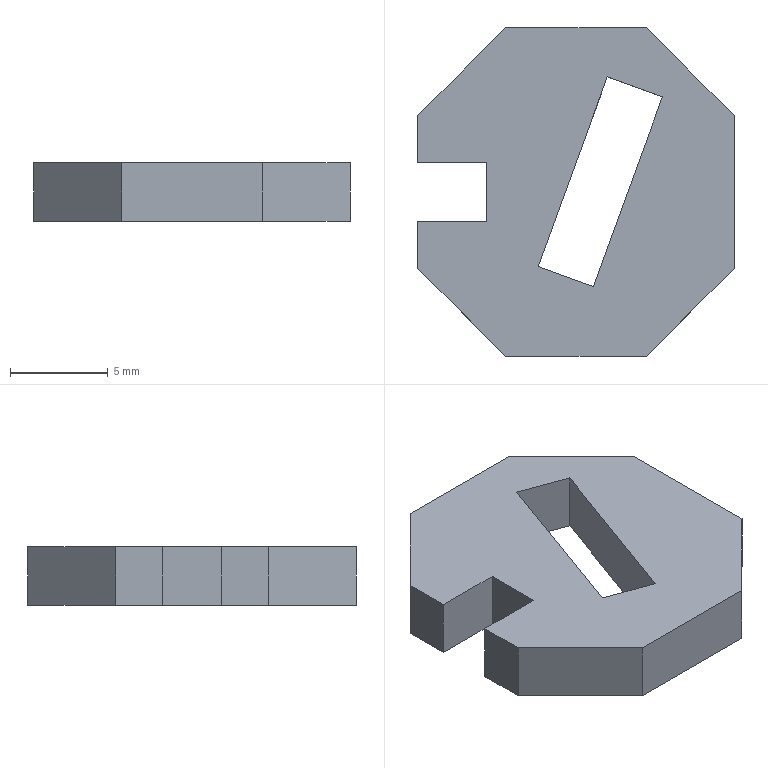Part | SolidWorks | features BaseBody 1 | 1 solid | 18 faces | box 16.185 x 16.813 x 3 mm | volume 570.375 mm3 | plane 18
STEP:
#1=CARTESIAN_POINT('',(11.966,25.62,-1.5));
#2=VERTEX_POINT('',#1);
#3=CARTESIAN_POINT('',(14.785,24.594,-1.5));
#4=VERTEX_POINT('',#3);
#5=CARTESIAN_POINT('',(14.785,24.594,-1.5));
#6=DIRECTION('',(0.9396,-0.3421,0.));
#7=VECTOR('',#6,1000.);
#8=LINE('',#5,#7);
#9=EDGE_CURVE('',#2,#4,#8,.T.);
#10=ORIENTED_EDGE('',*,*,#9,.F.);
#11=CARTESIAN_POINT('',(11.966,25.62,1.5));
#12=VERTEX_POINT('',#11);
#13=CARTESIAN_POINT('',(11.966,25.62,1.5));
#14=DIRECTION('',(0.,0.,-1.));
#15=VECTOR('',#14,1000.);
#16=LINE('',#13,#15);
#17=EDGE_CURVE('',#12,#2,#16,.T.);
#18=ORIENTED_EDGE('',*,*,#17,.F.);
#19=CARTESIAN_POINT('',(14.785,24.594,1.5));
#20=VERTEX_POINT('',#19);
#21=CARTESIAN_POINT('',(14.785,24.594,1.5));
#22=DIRECTION('',(0.9396,-0.3421,0.));
#23=VECTOR('',#22,1000.);
#24=LINE('',#21,#23);
#25=EDGE_CURVE('',#12,#20,#24,.T.);
#26=ORIENTED_EDGE('',*,*,#25,.T.);
#27=CARTESIAN_POINT('',(14.785,24.594,1.5));
#28=DIRECTION('',(0.,0.,-1.));
#29=VECTOR('',#28,1000.);
#30=LINE('',#27,#29);
#31=EDGE_CURVE('',#20,#4,#30,.T.);
#32=ORIENTED_EDGE('',*,*,#31,.T.);
#33=EDGE_LOOP('',(#10,#18,#26,#32));
#34=FACE_OUTER_BOUND('',#33,.T.);
#35=CARTESIAN_POINT('',(14.785,24.594,1.5));
#36=DIRECTION('',(0.3421,0.9396,0.));
#37=DIRECTION('',(0.,0.,-1.));
#38=AXIS2_PLACEMENT_3D('',#35,#36,#37);
#39=PLANE('',#38);
#40=ADVANCED_FACE('',(#34),#39,.T.);
#41=CARTESIAN_POINT('',(15.5,35.326,-1.5));
#42=VERTEX_POINT('',#41);
#43=CARTESIAN_POINT('',(11.966,25.62,-1.5));
#44=DIRECTION('',(-0.3421,-0.9396,0.));
#45=VECTOR('',#44,1000.);
#46=LINE('',#43,#45);
#47=EDGE_CURVE('',#42,#2,#46,.T.);
#48=ORIENTED_EDGE('',*,*,#47,.F.);
#49=CARTESIAN_POINT('',(15.5,35.326,1.5));
#50=VERTEX_POINT('',#49);
#51=CARTESIAN_POINT('',(15.5,35.326,1.5));
#52=DIRECTION('',(0.,0.,-1.));
#53=VECTOR('',#52,1000.);
#54=LINE('',#51,#53);
#55=EDGE_CURVE('',#50,#42,#54,.T.);
#56=ORIENTED_EDGE('',*,*,#55,.F.);
#57=CARTESIAN_POINT('',(11.966,25.62,1.5));
#58=DIRECTION('',(-0.3421,-0.9396,0.));
#59=VECTOR('',#58,1000.);
#60=LINE('',#57,#59);
#61=EDGE_CURVE('',#50,#12,#60,.T.);
#62=ORIENTED_EDGE('',*,*,#61,.T.);
#63=ORIENTED_EDGE('',*,*,#17,.T.);
#64=EDGE_LOOP('',(#48,#56,#62,#63));
#65=FACE_OUTER_BOUND('',#64,.T.);
#66=CARTESIAN_POINT('',(11.966,25.62,1.5));
#67=DIRECTION('',(0.9396,-0.3421,0.));
#68=DIRECTION('',(0.,0.,-1.));
#69=AXIS2_PLACEMENT_3D('',#66,#67,#68);
#70=PLANE('',#69);
#71=ADVANCED_FACE('',(#65),#70,.T.);
#72=CARTESIAN_POINT('',(18.319,34.3,-1.5));
#73=VERTEX_POINT('',#72);
#74=CARTESIAN_POINT('',(15.5,35.326,-1.5));
#75=DIRECTION('',(-0.9396,0.3421,0.));
#76=VECTOR('',#75,1000.);
#77=LINE('',#74,#76);
#78=EDGE_CURVE('',#73,#42,#77,.T.);
#79=ORIENTED_EDGE('',*,*,#78,.F.);
#80=CARTESIAN_POINT('',(18.319,34.3,1.5));
#81=VERTEX_POINT('',#80);
#82=CARTESIAN_POINT('',(18.319,34.3,1.5));
#83=DIRECTION('',(0.,0.,-1.));
#84=VECTOR('',#83,1000.);
#85=LINE('',#82,#84);
#86=EDGE_CURVE('',#81,#73,#85,.T.);
#87=ORIENTED_EDGE('',*,*,#86,.F.);
#88=CARTESIAN_POINT('',(15.5,35.326,1.5));
#89=DIRECTION('',(-0.9396,0.3421,0.));
#90=VECTOR('',#89,1000.);
#91=LINE('',#88,#90);
#92=EDGE_CURVE('',#81,#50,#91,.T.);
#93=ORIENTED_EDGE('',*,*,#92,.T.);
#94=ORIENTED_EDGE('',*,*,#55,.T.);
#95=EDGE_LOOP('',(#79,#87,#93,#94));
#96=FACE_OUTER_BOUND('',#95,.T.);
#97=CARTESIAN_POINT('',(15.5,35.326,1.5));
#98=DIRECTION('',(-0.3421,-0.9396,0.));
#99=DIRECTION('',(-0.9396,0.3421,0.));
#100=AXIS2_PLACEMENT_3D('',#97,#98,#99);
#101=PLANE('',#100);
#102=ADVANCED_FACE('',(#96),#101,.T.);
#103=CARTESIAN_POINT('',(18.319,34.3,-1.5));
#104=DIRECTION('',(0.3421,0.9396,0.));
#105=VECTOR('',#104,1000.);
#106=LINE('',#103,#105);
#107=EDGE_CURVE('',#4,#73,#106,.T.);
#108=ORIENTED_EDGE('',*,*,#107,.F.);
#109=ORIENTED_EDGE('',*,*,#31,.F.);
#110=CARTESIAN_POINT('',(18.319,34.3,1.5));
#111=DIRECTION('',(0.3421,0.9396,0.));
#112=VECTOR('',#111,1000.);
#113=LINE('',#110,#112);
#114=EDGE_CURVE('',#20,#81,#113,.T.);
#115=ORIENTED_EDGE('',*,*,#114,.T.);
#116=ORIENTED_EDGE('',*,*,#86,.T.);
#117=EDGE_LOOP('',(#108,#109,#115,#116));
#118=FACE_OUTER_BOUND('',#117,.T.);
#119=CARTESIAN_POINT('',(18.319,34.3,1.5));
#120=DIRECTION('',(-0.9396,0.3421,0.));
#121=DIRECTION('',(0.,0.,1.));
#122=AXIS2_PLACEMENT_3D('',#119,#120,#121);
#123=PLANE('',#122);
#124=ADVANCED_FACE('',(#118),#123,.T.);
#125=CARTESIAN_POINT('',(5.805,33.35,-1.5));
#126=VERTEX_POINT('',#125);
#127=CARTESIAN_POINT('',(5.805,30.942,-1.5));
#128=VERTEX_POINT('',#127);
#129=CARTESIAN_POINT('',(5.805,30.942,-1.5));
#130=DIRECTION('',(0.,-1.,0.));
#131=VECTOR('',#130,1000.);
#132=LINE('',#129,#131);
#133=EDGE_CURVE('',#126,#128,#132,.T.);
#134=ORIENTED_EDGE('',*,*,#133,.T.);
#135=CARTESIAN_POINT('',(5.805,30.942,1.5));
#136=VERTEX_POINT('',#135);
#137=CARTESIAN_POINT('',(5.805,30.942,1.5));
#138=DIRECTION('',(0.,0.,-1.));
#139=VECTOR('',#138,1000.);
#140=LINE('',#137,#139);
#141=EDGE_CURVE('',#136,#128,#140,.T.);
#142=ORIENTED_EDGE('',*,*,#141,.F.);
#143=CARTESIAN_POINT('',(5.805,33.35,1.5));
#144=VERTEX_POINT('',#143);
#145=CARTESIAN_POINT('',(5.805,30.942,1.5));
#146=DIRECTION('',(0.,-1.,0.));
#147=VECTOR('',#146,1000.);
#148=LINE('',#145,#147);
#149=EDGE_CURVE('',#144,#136,#148,.T.);
#150=ORIENTED_EDGE('',*,*,#149,.F.);
#151=CARTESIAN_POINT('',(5.805,33.35,1.5));
#152=DIRECTION('',(0.,0.,-1.));
#153=VECTOR('',#152,1000.);
#154=LINE('',#151,#153);
#155=EDGE_CURVE('',#144,#126,#154,.T.);
#156=ORIENTED_EDGE('',*,*,#155,.T.);
#157=EDGE_LOOP('',(#134,#142,#150,#156));
#158=FACE_OUTER_BOUND('',#157,.T.);
#159=CARTESIAN_POINT('',(5.805,30.942,1.5));
#160=DIRECTION('',(1.,0.,0.));
#161=DIRECTION('',(0.,1.,0.));
#162=AXIS2_PLACEMENT_3D('',#159,#160,#161);
#163=PLANE('',#162);
#164=ADVANCED_FACE('',(#158),#163,.F.);
#165=CARTESIAN_POINT('',(10.299,37.845,-1.5));
#166=VERTEX_POINT('',#165);
#167=CARTESIAN_POINT('',(5.805,33.35,-1.5));
#168=DIRECTION('',(-0.707,-0.7072,0.));
#169=VECTOR('',#168,1000.);
#170=LINE('',#167,#169);
#171=EDGE_CURVE('',#166,#126,#170,.T.);
#172=ORIENTED_EDGE('',*,*,#171,.T.);
#173=ORIENTED_EDGE('',*,*,#155,.F.);
#174=CARTESIAN_POINT('',(10.299,37.845,1.5));
#175=VERTEX_POINT('',#174);
#176=CARTESIAN_POINT('',(5.805,33.35,1.5));
#177=DIRECTION('',(-0.707,-0.7072,0.));
#178=VECTOR('',#177,1000.);
#179=LINE('',#176,#178);
#180=EDGE_CURVE('',#175,#144,#179,.T.);
#181=ORIENTED_EDGE('',*,*,#180,.F.);
#182=CARTESIAN_POINT('',(10.299,37.845,1.5));
#183=DIRECTION('',(0.,0.,-1.));
#184=VECTOR('',#183,1000.);
#185=LINE('',#182,#184);
#186=EDGE_CURVE('',#175,#166,#185,.T.);
#187=ORIENTED_EDGE('',*,*,#186,.T.);
#188=EDGE_LOOP('',(#172,#173,#181,#187));
#189=FACE_OUTER_BOUND('',#188,.T.);
#190=CARTESIAN_POINT('',(5.805,33.35,1.5));
#191=DIRECTION('',(0.7072,-0.707,0.));
#192=DIRECTION('',(0.,0.,-1.));
#193=AXIS2_PLACEMENT_3D('',#190,#191,#192);
#194=PLANE('',#193);
#195=ADVANCED_FACE('',(#189),#194,.F.);
#196=CARTESIAN_POINT('',(17.494,37.845,-1.5));
#197=VERTEX_POINT('',#196);
#198=CARTESIAN_POINT('',(10.299,37.845,-1.5));
#199=DIRECTION('',(-1.,0.,0.));
#200=VECTOR('',#199,1000.);
#201=LINE('',#198,#200);
#202=EDGE_CURVE('',#197,#166,#201,.T.);
#203=ORIENTED_EDGE('',*,*,#202,.T.);
#204=ORIENTED_EDGE('',*,*,#186,.F.);
#205=CARTESIAN_POINT('',(17.494,37.845,1.5));
#206=VERTEX_POINT('',#205);
#207=CARTESIAN_POINT('',(10.299,37.845,1.5));
#208=DIRECTION('',(-1.,0.,0.));
#209=VECTOR('',#208,1000.);
#210=LINE('',#207,#209);
#211=EDGE_CURVE('',#206,#175,#210,.T.);
#212=ORIENTED_EDGE('',*,*,#211,.F.);
#213=CARTESIAN_POINT('',(17.494,37.845,1.5));
#214=DIRECTION('',(0.,0.,-1.));
#215=VECTOR('',#214,1000.);
#216=LINE('',#213,#215);
#217=EDGE_CURVE('',#206,#197,#216,.T.);
#218=ORIENTED_EDGE('',*,*,#217,.T.);
#219=EDGE_LOOP('',(#203,#204,#212,#218));
#220=FACE_OUTER_BOUND('',#219,.T.);
#221=CARTESIAN_POINT('',(10.299,37.845,1.5));
#222=DIRECTION('',(0.,-1.,0.));
#223=DIRECTION('',(0.,0.,-1.));
#224=AXIS2_PLACEMENT_3D('',#221,#222,#223);
#225=PLANE('',#224);
#226=ADVANCED_FACE('',(#220),#225,.F.);
#227=CARTESIAN_POINT('',(21.99,33.35,-1.5));
#228=VERTEX_POINT('',#227);
#229=CARTESIAN_POINT('',(17.494,37.845,-1.5));
#230=DIRECTION('',(-0.7071,0.7071,0.));
#231=VECTOR('',#230,1000.);
#232=LINE('',#229,#231);
#233=EDGE_CURVE('',#228,#197,#232,.T.);
#234=ORIENTED_EDGE('',*,*,#233,.T.);
#235=ORIENTED_EDGE('',*,*,#217,.F.);
#236=CARTESIAN_POINT('',(21.99,33.35,1.5));
#237=VERTEX_POINT('',#236);
#238=CARTESIAN_POINT('',(17.494,37.845,1.5));
#239=DIRECTION('',(-0.7071,0.7071,0.));
#240=VECTOR('',#239,1000.);
#241=LINE('',#238,#240);
#242=EDGE_CURVE('',#237,#206,#241,.T.);
#243=ORIENTED_EDGE('',*,*,#242,.F.);
#244=CARTESIAN_POINT('',(21.99,33.35,1.5));
#245=DIRECTION('',(0.,0.,-1.));
#246=VECTOR('',#245,1000.);
#247=LINE('',#244,#246);
#248=EDGE_CURVE('',#237,#228,#247,.T.);
#249=ORIENTED_EDGE('',*,*,#248,.T.);
#250=EDGE_LOOP('',(#234,#235,#243,#249));
#251=FACE_OUTER_BOUND('',#250,.T.);
#252=CARTESIAN_POINT('',(17.494,37.845,1.5));
#253=DIRECTION('',(-0.7071,-0.7071,0.));
#254=DIRECTION('',(-0.7071,0.7071,0.));
#255=AXIS2_PLACEMENT_3D('',#252,#253,#254);
#256=PLANE('',#255);
#257=ADVANCED_FACE('',(#251),#256,.F.);
#258=CARTESIAN_POINT('',(21.99,25.525,-1.5));
#259=VERTEX_POINT('',#258);
#260=CARTESIAN_POINT('',(21.99,33.35,-1.5));
#261=DIRECTION('',(0.,1.,0.));
#262=VECTOR('',#261,1000.);
#263=LINE('',#260,#262);
#264=EDGE_CURVE('',#259,#228,#263,.T.);
#265=ORIENTED_EDGE('',*,*,#264,.T.);
#266=ORIENTED_EDGE('',*,*,#248,.F.);
#267=CARTESIAN_POINT('',(21.99,25.525,1.5));
#268=VERTEX_POINT('',#267);
#269=CARTESIAN_POINT('',(21.99,33.35,1.5));
#270=DIRECTION('',(0.,1.,0.));
#271=VECTOR('',#270,1000.);
#272=LINE('',#269,#271);
#273=EDGE_CURVE('',#268,#237,#272,.T.);
#274=ORIENTED_EDGE('',*,*,#273,.F.);
#275=CARTESIAN_POINT('',(21.99,25.525,1.5));
#276=DIRECTION('',(0.,0.,-1.));
#277=VECTOR('',#276,1000.);
#278=LINE('',#275,#277);
#279=EDGE_CURVE('',#268,#259,#278,.T.);
#280=ORIENTED_EDGE('',*,*,#279,.T.);
#281=EDGE_LOOP('',(#265,#266,#274,#280));
#282=FACE_OUTER_BOUND('',#281,.T.);
#283=CARTESIAN_POINT('',(21.99,33.35,1.5));
#284=DIRECTION('',(-1.,0.,0.));
#285=DIRECTION('',(0.,0.,1.));
#286=AXIS2_PLACEMENT_3D('',#283,#284,#285);
#287=PLANE('',#286);
#288=ADVANCED_FACE('',(#282),#287,.F.);
#289=CARTESIAN_POINT('',(17.494,21.033,-1.5));
#290=VERTEX_POINT('',#289);
#291=CARTESIAN_POINT('',(21.99,25.525,-1.5));
#292=DIRECTION('',(0.7073,0.7069,0.));
#293=VECTOR('',#292,1000.);
#294=LINE('',#291,#293);
#295=EDGE_CURVE('',#290,#259,#294,.T.);
#296=ORIENTED_EDGE('',*,*,#295,.T.);
#297=ORIENTED_EDGE('',*,*,#279,.F.);
#298=CARTESIAN_POINT('',(17.494,21.033,1.5));
#299=VERTEX_POINT('',#298);
#300=CARTESIAN_POINT('',(21.99,25.525,1.5));
#301=DIRECTION('',(0.7073,0.7069,0.));
#302=VECTOR('',#301,1000.);
#303=LINE('',#300,#302);
#304=EDGE_CURVE('',#299,#268,#303,.T.);
#305=ORIENTED_EDGE('',*,*,#304,.F.);
#306=CARTESIAN_POINT('',(17.494,21.033,1.5));
#307=DIRECTION('',(0.,0.,-1.));
#308=VECTOR('',#307,1000.);
#309=LINE('',#306,#308);
#310=EDGE_CURVE('',#299,#290,#309,.T.);
#311=ORIENTED_EDGE('',*,*,#310,.T.);
#312=EDGE_LOOP('',(#296,#297,#305,#311));
#313=FACE_OUTER_BOUND('',#312,.T.);
#314=CARTESIAN_POINT('',(21.99,25.525,1.5));
#315=DIRECTION('',(-0.7069,0.7073,0.));
#316=DIRECTION('',(0.,0.,1.));
#317=AXIS2_PLACEMENT_3D('',#314,#315,#316);
#318=PLANE('',#317);
#319=ADVANCED_FACE('',(#313),#318,.F.);
#320=CARTESIAN_POINT('',(10.299,21.033,-1.5));
#321=VERTEX_POINT('',#320);
#322=CARTESIAN_POINT('',(17.494,21.033,-1.5));
#323=DIRECTION('',(1.,0.,0.));
#324=VECTOR('',#323,1000.);
#325=LINE('',#322,#324);
#326=EDGE_CURVE('',#321,#290,#325,.T.);
#327=ORIENTED_EDGE('',*,*,#326,.T.);
#328=ORIENTED_EDGE('',*,*,#310,.F.);
#329=CARTESIAN_POINT('',(10.299,21.033,1.5));
#330=VERTEX_POINT('',#329);
#331=CARTESIAN_POINT('',(17.494,21.033,1.5));
#332=DIRECTION('',(1.,0.,0.));
#333=VECTOR('',#332,1000.);
#334=LINE('',#331,#333);
#335=EDGE_CURVE('',#330,#299,#334,.T.);
#336=ORIENTED_EDGE('',*,*,#335,.F.);
#337=CARTESIAN_POINT('',(10.299,21.033,1.5));
#338=DIRECTION('',(0.,0.,-1.));
#339=VECTOR('',#338,1000.);
#340=LINE('',#337,#339);
#341=EDGE_CURVE('',#330,#321,#340,.T.);
#342=ORIENTED_EDGE('',*,*,#341,.T.);
#343=EDGE_LOOP('',(#327,#328,#336,#342));
#344=FACE_OUTER_BOUND('',#343,.T.);
#345=CARTESIAN_POINT('',(17.494,21.033,1.5));
#346=DIRECTION('',(0.,1.,0.));
#347=DIRECTION('',(1.,0.,0.));
#348=AXIS2_PLACEMENT_3D('',#345,#346,#347);
#349=PLANE('',#348);
#350=ADVANCED_FACE('',(#344),#349,.F.);
#351=CARTESIAN_POINT('',(5.805,25.525,-1.5));
#352=VERTEX_POINT('',#351);
#353=CARTESIAN_POINT('',(10.299,21.033,-1.5));
#354=DIRECTION('',(0.7073,-0.7069,0.));
#355=VECTOR('',#354,1000.);
#356=LINE('',#353,#355);
#357=EDGE_CURVE('',#352,#321,#356,.T.);
#358=ORIENTED_EDGE('',*,*,#357,.T.);
#359=ORIENTED_EDGE('',*,*,#341,.F.);
#360=CARTESIAN_POINT('',(5.805,25.525,1.5));
#361=VERTEX_POINT('',#360);
#362=CARTESIAN_POINT('',(10.299,21.033,1.5));
#363=DIRECTION('',(0.7073,-0.7069,0.));
#364=VECTOR('',#363,1000.);
#365=LINE('',#362,#364);
#366=EDGE_CURVE('',#361,#330,#365,.T.);
#367=ORIENTED_EDGE('',*,*,#366,.F.);
#368=CARTESIAN_POINT('',(5.805,25.525,1.5));
#369=DIRECTION('',(0.,0.,-1.));
#370=VECTOR('',#369,1000.);
#371=LINE('',#368,#370);
#372=EDGE_CURVE('',#361,#352,#371,.T.);
#373=ORIENTED_EDGE('',*,*,#372,.T.);
#374=EDGE_LOOP('',(#358,#359,#367,#373));
#375=FACE_OUTER_BOUND('',#374,.T.);
#376=CARTESIAN_POINT('',(10.299,21.033,1.5));
#377=DIRECTION('',(0.7069,0.7073,0.));
#378=DIRECTION('',(0.,0.,-1.));
#379=AXIS2_PLACEMENT_3D('',#376,#377,#378);
#380=PLANE('',#379);
#381=ADVANCED_FACE('',(#375),#380,.F.);
#382=CARTESIAN_POINT('',(5.805,27.942,-1.5));
#383=VERTEX_POINT('',#382);
#384=CARTESIAN_POINT('',(5.805,25.525,-1.5));
#385=DIRECTION('',(0.,-1.,0.));
#386=VECTOR('',#385,1000.);
#387=LINE('',#384,#386);
#388=EDGE_CURVE('',#383,#352,#387,.T.);
#389=ORIENTED_EDGE('',*,*,#388,.T.);
#390=ORIENTED_EDGE('',*,*,#372,.F.);
#391=CARTESIAN_POINT('',(5.805,27.942,1.5));
#392=VERTEX_POINT('',#391);
#393=CARTESIAN_POINT('',(5.805,25.525,1.5));
#394=DIRECTION('',(0.,-1.,0.));
#395=VECTOR('',#394,1000.);
#396=LINE('',#393,#395);
#397=EDGE_CURVE('',#392,#361,#396,.T.);
#398=ORIENTED_EDGE('',*,*,#397,.F.);
#399=CARTESIAN_POINT('',(5.805,27.942,1.5));
#400=DIRECTION('',(0.,0.,-1.));
#401=VECTOR('',#400,1000.);
#402=LINE('',#399,#401);
#403=EDGE_CURVE('',#392,#383,#402,.T.);
#404=ORIENTED_EDGE('',*,*,#403,.T.);
#405=EDGE_LOOP('',(#389,#390,#398,#404));
#406=FACE_OUTER_BOUND('',#405,.T.);
#407=CARTESIAN_POINT('',(5.805,25.525,1.5));
#408=DIRECTION('',(1.,0.,0.));
#409=DIRECTION('',(0.,1.,0.));
#410=AXIS2_PLACEMENT_3D('',#407,#408,#409);
#411=PLANE('',#410);
#412=ADVANCED_FACE('',(#406),#411,.F.);
#413=CARTESIAN_POINT('',(9.34,27.942,-1.5));
#414=VERTEX_POINT('',#413);
#415=CARTESIAN_POINT('',(5.805,27.942,-1.5));
#416=DIRECTION('',(-1.,0.,0.));
#417=VECTOR('',#416,1000.);
#418=LINE('',#415,#417);
#419=EDGE_CURVE('',#414,#383,#418,.T.);
#420=ORIENTED_EDGE('',*,*,#419,.T.);
#421=ORIENTED_EDGE('',*,*,#403,.F.);
#422=CARTESIAN_POINT('',(9.34,27.942,1.5));
#423=VERTEX_POINT('',#422);
#424=CARTESIAN_POINT('',(5.805,27.942,1.5));
#425=DIRECTION('',(-1.,0.,0.));
#426=VECTOR('',#425,1000.);
#427=LINE('',#424,#426);
#428=EDGE_CURVE('',#423,#392,#427,.T.);
#429=ORIENTED_EDGE('',*,*,#428,.F.);
#430=CARTESIAN_POINT('',(9.34,27.942,1.5));
#431=DIRECTION('',(0.,0.,-1.));
#432=VECTOR('',#431,1000.);
#433=LINE('',#430,#432);
#434=EDGE_CURVE('',#423,#414,#433,.T.);
#435=ORIENTED_EDGE('',*,*,#434,.T.);
#436=EDGE_LOOP('',(#420,#421,#429,#435));
#437=FACE_OUTER_BOUND('',#436,.T.);
#438=CARTESIAN_POINT('',(5.805,27.942,1.5));
#439=DIRECTION('',(0.,-1.,0.));
#440=DIRECTION('',(0.,0.,-1.));
#441=AXIS2_PLACEMENT_3D('',#438,#439,#440);
#442=PLANE('',#441);
#443=ADVANCED_FACE('',(#437),#442,.F.);
#444=CARTESIAN_POINT('',(9.34,30.942,-1.5));
#445=VERTEX_POINT('',#444);
#446=CARTESIAN_POINT('',(9.34,27.942,-1.5));
#447=DIRECTION('',(0.,-1.,0.));
#448=VECTOR('',#447,1000.);
#449=LINE('',#446,#448);
#450=EDGE_CURVE('',#445,#414,#449,.T.);
#451=ORIENTED_EDGE('',*,*,#450,.T.);
#452=ORIENTED_EDGE('',*,*,#434,.F.);
#453=CARTESIAN_POINT('',(9.34,30.942,1.5));
#454=VERTEX_POINT('',#453);
#455=CARTESIAN_POINT('',(9.34,27.942,1.5));
#456=DIRECTION('',(0.,-1.,0.));
#457=VECTOR('',#456,1000.);
#458=LINE('',#455,#457);
#459=EDGE_CURVE('',#454,#423,#458,.T.);
#460=ORIENTED_EDGE('',*,*,#459,.F.);
#461=CARTESIAN_POINT('',(9.34,30.942,1.5));
#462=DIRECTION('',(0.,0.,-1.));
#463=VECTOR('',#462,1000.);
#464=LINE('',#461,#463);
#465=EDGE_CURVE('',#454,#445,#464,.T.);
#466=ORIENTED_EDGE('',*,*,#465,.T.);
#467=EDGE_LOOP('',(#451,#452,#460,#466));
#468=FACE_OUTER_BOUND('',#467,.T.);
#469=CARTESIAN_POINT('',(9.34,27.942,1.5));
#470=DIRECTION('',(1.,0.,0.));
#471=DIRECTION('',(0.,1.,0.));
#472=AXIS2_PLACEMENT_3D('',#469,#470,#471);
#473=PLANE('',#472);
#474=ADVANCED_FACE('',(#468),#473,.F.);
#475=CARTESIAN_POINT('',(9.34,30.942,-1.5));
#476=DIRECTION('',(1.,0.,0.));
#477=VECTOR('',#476,1000.);
#478=LINE('',#475,#477);
#479=EDGE_CURVE('',#128,#445,#478,.T.);
#480=ORIENTED_EDGE('',*,*,#479,.T.);
#481=ORIENTED_EDGE('',*,*,#465,.F.);
#482=CARTESIAN_POINT('',(9.34,30.942,1.5));
#483=DIRECTION('',(1.,0.,0.));
#484=VECTOR('',#483,1000.);
#485=LINE('',#482,#484);
#486=EDGE_CURVE('',#136,#454,#485,.T.);
#487=ORIENTED_EDGE('',*,*,#486,.F.);
#488=ORIENTED_EDGE('',*,*,#141,.T.);
#489=EDGE_LOOP('',(#480,#481,#487,#488));
#490=FACE_OUTER_BOUND('',#489,.T.);
#491=CARTESIAN_POINT('',(9.34,30.942,1.5));
#492=DIRECTION('',(0.,1.,0.));
#493=DIRECTION('',(1.,0.,0.));
#494=AXIS2_PLACEMENT_3D('',#491,#492,#493);
#495=PLANE('',#494);
#496=ADVANCED_FACE('',(#490),#495,.F.);
#497=ORIENTED_EDGE('',*,*,#9,.T.);
#498=ORIENTED_EDGE('',*,*,#107,.T.);
#499=ORIENTED_EDGE('',*,*,#78,.T.);
#500=ORIENTED_EDGE('',*,*,#47,.T.);
#501=EDGE_LOOP('',(#497,#498,#499,#500));
#502=FACE_BOUND('',#501,.T.);
#503=ORIENTED_EDGE('',*,*,#479,.F.);
#504=ORIENTED_EDGE('',*,*,#133,.F.);
#505=ORIENTED_EDGE('',*,*,#171,.F.);
#506=ORIENTED_EDGE('',*,*,#202,.F.);
#507=ORIENTED_EDGE('',*,*,#233,.F.);
#508=ORIENTED_EDGE('',*,*,#264,.F.);
#509=ORIENTED_EDGE('',*,*,#295,.F.);
#510=ORIENTED_EDGE('',*,*,#326,.F.);
#511=ORIENTED_EDGE('',*,*,#357,.F.);
#512=ORIENTED_EDGE('',*,*,#388,.F.);
#513=ORIENTED_EDGE('',*,*,#419,.F.);
#514=ORIENTED_EDGE('',*,*,#450,.F.);
#515=EDGE_LOOP('',(#503,#504,#505,#506,#507,#508,#509,#510,#511,#512,#513,#514));
#516=FACE_OUTER_BOUND('',#515,.T.);
#517=CARTESIAN_POINT('',(0.,0.,-1.5));
#518=DIRECTION('',(0.,0.,-1.));
#519=DIRECTION('',(0.,-1.,0.));
#520=AXIS2_PLACEMENT_3D('',#517,#518,#519);
#521=PLANE('',#520);
#522=ADVANCED_FACE('',(#502,#516),#521,.T.);
#523=ORIENTED_EDGE('',*,*,#114,.F.);
#524=ORIENTED_EDGE('',*,*,#25,.F.);
#525=ORIENTED_EDGE('',*,*,#61,.F.);
#526=ORIENTED_EDGE('',*,*,#92,.F.);
#527=EDGE_LOOP('',(#523,#524,#525,#526));
#528=FACE_BOUND('',#527,.T.);
#529=ORIENTED_EDGE('',*,*,#486,.T.);
#530=ORIENTED_EDGE('',*,*,#459,.T.);
#531=ORIENTED_EDGE('',*,*,#428,.T.);
#532=ORIENTED_EDGE('',*,*,#397,.T.);
#533=ORIENTED_EDGE('',*,*,#366,.T.);
#534=ORIENTED_EDGE('',*,*,#335,.T.);
#535=ORIENTED_EDGE('',*,*,#304,.T.);
#536=ORIENTED_EDGE('',*,*,#273,.T.);
#537=ORIENTED_EDGE('',*,*,#242,.T.);
#538=ORIENTED_EDGE('',*,*,#211,.T.);
#539=ORIENTED_EDGE('',*,*,#180,.T.);
#540=ORIENTED_EDGE('',*,*,#149,.T.);
#541=EDGE_LOOP('',(#529,#530,#531,#532,#533,#534,#535,#536,#537,#538,#539,#540));
#542=FACE_OUTER_BOUND('',#541,.T.);
#543=CARTESIAN_POINT('',(0.,0.,1.5));
#544=DIRECTION('',(0.,0.,-1.));
#545=DIRECTION('',(0.,-1.,0.));
#546=AXIS2_PLACEMENT_3D('',#543,#544,#545);
#547=PLANE('',#546);
#548=ADVANCED_FACE('',(#528,#542),#547,.F.);
#549=CLOSED_SHELL('',(#40,#71,#102,#124,#164,#195,#226,#257,#288,#319,#350,#381,#412,#443,#474,#496,#522,#548));
#550=MANIFOLD_SOLID_BREP('',#549);
#551=CARTESIAN_POINT('',(0.,0.,0.));
#552=DIRECTION('',(0.,0.,1.));
#553=DIRECTION('',(1.,0.,0.));
#554=AXIS2_PLACEMENT_3D('',#551,#552,#553);
#555=(LENGTH_UNIT()NAMED_UNIT(*)SI_UNIT(.MILLI.,.METRE.));
#556=UNCERTAINTY_MEASURE_WITH_UNIT(LENGTH_MEASURE(0.00001),#555,'','');
#557=(NAMED_UNIT(*)PLANE_ANGLE_UNIT()SI_UNIT($,.RADIAN.));
#558=(NAMED_UNIT(*)SI_UNIT($,.STERADIAN.)SOLID_ANGLE_UNIT());
#559=(GEOMETRIC_REPRESENTATION_CONTEXT(3)GLOBAL_UNCERTAINTY_ASSIGNED_CONTEXT((#556))GLOBAL_UNIT_ASSIGNED_CONTEXT((#555,#557,#558))REPRESENTATION_CONTEXT('',''));
#560=ADVANCED_BREP_SHAPE_REPRESENTATION('',(#550,#554),#559);